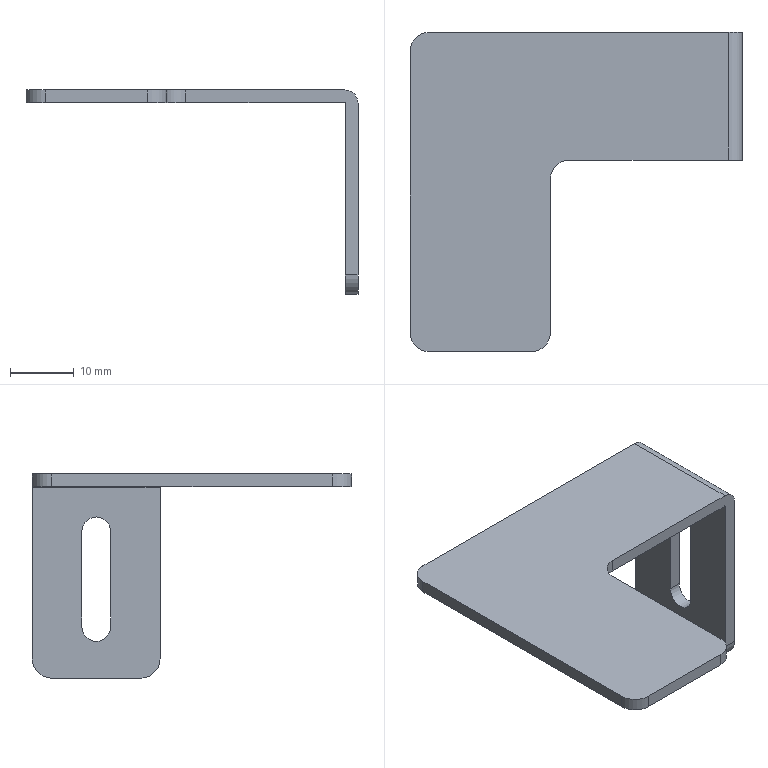Part | SolidWorks | features Fillet 2, Cut 1, FlatPattern 1, ICE 1, SMBaseFlange 1, SheetMetal 1 | 1 solid | 25 faces | box 52 x 50 x 32 mm | volume 4399 mm3 | plane 14 | cylinder 11 | commonest cylinder face diameters 6 x6 4.5 x3 0.2 x1 4.2 x1
STEP:
#1=CARTESIAN_POINT('',(52.,40.,-4.75));
#2=VERTEX_POINT('',#1);
#3=CARTESIAN_POINT('',(52.,42.25,-7.));
#4=VERTEX_POINT('',#3);
#5=CARTESIAN_POINT('',(52.,40.,-7.));
#6=DIRECTION('',(-1.,0.,0.));
#7=DIRECTION('',(0.,0.,1.));
#8=AXIS2_PLACEMENT_3D('',#5,#6,#7);
#9=CIRCLE('',#8,2.25);
#10=EDGE_CURVE('',#2,#4,#9,.T.);
#11=ORIENTED_EDGE('',*,*,#10,.F.);
#12=CARTESIAN_POINT('',(50.,40.,-4.75));
#13=VERTEX_POINT('',#12);
#14=CARTESIAN_POINT('',(52.,40.,-4.75));
#15=DIRECTION('',(-1.,0.,0.));
#16=VECTOR('',#15,1000.);
#17=LINE('',#14,#16);
#18=EDGE_CURVE('',#2,#13,#17,.T.);
#19=ORIENTED_EDGE('',*,*,#18,.T.);
#20=CARTESIAN_POINT('',(50.,42.25,-7.));
#21=VERTEX_POINT('',#20);
#22=CARTESIAN_POINT('',(50.,40.,-7.));
#23=DIRECTION('',(-1.,0.,0.));
#24=DIRECTION('',(0.,0.,1.));
#25=AXIS2_PLACEMENT_3D('',#22,#23,#24);
#26=CIRCLE('',#25,2.25);
#27=EDGE_CURVE('',#13,#21,#26,.T.);
#28=ORIENTED_EDGE('',*,*,#27,.T.);
#29=CARTESIAN_POINT('',(52.,42.25,-7.));
#30=DIRECTION('',(-1.,0.,0.));
#31=VECTOR('',#30,1000.);
#32=LINE('',#29,#31);
#33=EDGE_CURVE('',#4,#21,#32,.T.);
#34=ORIENTED_EDGE('',*,*,#33,.F.);
#35=EDGE_LOOP('',(#11,#19,#28,#34));
#36=FACE_OUTER_BOUND('',#35,.T.);
#37=CARTESIAN_POINT('',(52.,40.,-7.));
#38=DIRECTION('',(-1.,0.,0.));
#39=DIRECTION('',(0.,0.,1.));
#40=AXIS2_PLACEMENT_3D('',#37,#38,#39);
#41=CYLINDRICAL_SURFACE('',#40,2.25);
#42=ADVANCED_FACE('',(#36),#41,.F.);
#43=CARTESIAN_POINT('',(50.,50.,-0.1));
#44=VERTEX_POINT('',#43);
#45=CARTESIAN_POINT('',(52.,50.,-0.1));
#46=VERTEX_POINT('',#45);
#47=CARTESIAN_POINT('',(50.,50.,-0.1));
#48=DIRECTION('',(1.,0.,0.));
#49=VECTOR('',#48,1000.);
#50=LINE('',#47,#49);
#51=EDGE_CURVE('',#44,#46,#50,.T.);
#52=ORIENTED_EDGE('',*,*,#51,.F.);
#53=CARTESIAN_POINT('',(49.9,50.,0.));
#54=VERTEX_POINT('',#53);
#55=CARTESIAN_POINT('',(49.9,50.,-0.1));
#56=DIRECTION('',(0.,1.,0.));
#57=DIRECTION('',(0.,0.,-1.));
#58=AXIS2_PLACEMENT_3D('',#55,#56,#57);
#59=CIRCLE('',#58,0.1);
#60=EDGE_CURVE('',#54,#44,#59,.T.);
#61=ORIENTED_EDGE('',*,*,#60,.F.);
#62=CARTESIAN_POINT('',(49.9,50.,2.));
#63=VERTEX_POINT('',#62);
#64=CARTESIAN_POINT('',(49.9,50.,2.));
#65=DIRECTION('',(0.,0.,-1.));
#66=VECTOR('',#65,1000.);
#67=LINE('',#64,#66);
#68=EDGE_CURVE('',#63,#54,#67,.T.);
#69=ORIENTED_EDGE('',*,*,#68,.F.);
#70=CARTESIAN_POINT('',(49.9,50.,-0.1));
#71=DIRECTION('',(0.,1.,0.));
#72=DIRECTION('',(1.,0.,0.));
#73=AXIS2_PLACEMENT_3D('',#70,#71,#72);
#74=CIRCLE('',#73,2.1);
#75=EDGE_CURVE('',#63,#46,#74,.T.);
#76=ORIENTED_EDGE('',*,*,#75,.T.);
#77=EDGE_LOOP('',(#52,#61,#69,#76));
#78=FACE_OUTER_BOUND('',#77,.T.);
#79=CARTESIAN_POINT('',(50.,50.,-0.1));
#80=DIRECTION('',(0.,1.,0.));
#81=DIRECTION('',(0.,0.,1.));
#82=AXIS2_PLACEMENT_3D('',#79,#80,#81);
#83=PLANE('',#82);
#84=ADVANCED_FACE('',(#78),#83,.T.);
#85=CARTESIAN_POINT('',(52.,50.,-27.));
#86=VERTEX_POINT('',#85);
#87=CARTESIAN_POINT('',(52.,50.,0.));
#88=DIRECTION('',(0.,0.,-1.));
#89=VECTOR('',#88,1000.);
#90=LINE('',#87,#89);
#91=EDGE_CURVE('',#46,#86,#90,.T.);
#92=ORIENTED_EDGE('',*,*,#91,.T.);
#93=CARTESIAN_POINT('',(50.,50.,-27.));
#94=VERTEX_POINT('',#93);
#95=CARTESIAN_POINT('',(49.9,50.,-27.));
#96=DIRECTION('',(-1.,0.,0.));
#97=VECTOR('',#96,1000.);
#98=LINE('',#95,#97);
#99=EDGE_CURVE('',#86,#94,#98,.T.);
#100=ORIENTED_EDGE('',*,*,#99,.T.);
#101=CARTESIAN_POINT('',(50.,50.,0.));
#102=DIRECTION('',(0.,0.,-1.));
#103=VECTOR('',#102,1000.);
#104=LINE('',#101,#103);
#105=EDGE_CURVE('',#44,#94,#104,.T.);
#106=ORIENTED_EDGE('',*,*,#105,.F.);
#107=ORIENTED_EDGE('',*,*,#51,.T.);
#108=EDGE_LOOP('',(#92,#100,#106,#107));
#109=FACE_OUTER_BOUND('',#108,.T.);
#110=CARTESIAN_POINT('',(49.9,50.,2.));
#111=DIRECTION('',(0.,1.,0.));
#112=DIRECTION('',(0.,0.,1.));
#113=AXIS2_PLACEMENT_3D('',#110,#111,#112);
#114=PLANE('',#113);
#115=ADVANCED_FACE('',(#109),#114,.T.);
#116=CARTESIAN_POINT('',(3.,0.,0.));
#117=VERTEX_POINT('',#116);
#118=CARTESIAN_POINT('',(19.,0.,0.));
#119=VERTEX_POINT('',#118);
#120=CARTESIAN_POINT('',(0.,0.,0.));
#121=DIRECTION('',(1.,0.,0.));
#122=VECTOR('',#121,1000.);
#123=LINE('',#120,#122);
#124=EDGE_CURVE('',#117,#119,#123,.T.);
#125=ORIENTED_EDGE('',*,*,#124,.T.);
#126=CARTESIAN_POINT('',(19.,0.,2.));
#127=VERTEX_POINT('',#126);
#128=CARTESIAN_POINT('',(19.,0.,2.));
#129=DIRECTION('',(0.,0.,1.));
#130=VECTOR('',#129,1000.);
#131=LINE('',#128,#130);
#132=EDGE_CURVE('',#119,#127,#131,.T.);
#133=ORIENTED_EDGE('',*,*,#132,.T.);
#134=CARTESIAN_POINT('',(3.,0.,2.));
#135=VERTEX_POINT('',#134);
#136=CARTESIAN_POINT('',(0.,0.,2.));
#137=DIRECTION('',(1.,0.,0.));
#138=VECTOR('',#137,1000.);
#139=LINE('',#136,#138);
#140=EDGE_CURVE('',#135,#127,#139,.T.);
#141=ORIENTED_EDGE('',*,*,#140,.F.);
#142=CARTESIAN_POINT('',(3.,0.,-0.1));
#143=DIRECTION('',(0.,0.,-1.));
#144=VECTOR('',#143,1000.);
#145=LINE('',#142,#144);
#146=EDGE_CURVE('',#135,#117,#145,.T.);
#147=ORIENTED_EDGE('',*,*,#146,.T.);
#148=EDGE_LOOP('',(#125,#133,#141,#147));
#149=FACE_OUTER_BOUND('',#148,.T.);
#150=CARTESIAN_POINT('',(52.,0.,-0.1));
#151=DIRECTION('',(0.,-1.,0.));
#152=DIRECTION('',(0.,0.,-1.));
#153=AXIS2_PLACEMENT_3D('',#150,#151,#152);
#154=PLANE('',#153);
#155=ADVANCED_FACE('',(#149),#154,.T.);
#156=CARTESIAN_POINT('',(52.,37.75,-22.));
#157=VERTEX_POINT('',#156);
#158=CARTESIAN_POINT('',(52.,37.75,-7.));
#159=VERTEX_POINT('',#158);
#160=CARTESIAN_POINT('',(52.,37.75,-7.));
#161=DIRECTION('',(0.,0.,1.));
#162=VECTOR('',#161,1000.);
#163=LINE('',#160,#162);
#164=EDGE_CURVE('',#157,#159,#163,.T.);
#165=ORIENTED_EDGE('',*,*,#164,.T.);
#166=CARTESIAN_POINT('',(52.,40.,-7.));
#167=DIRECTION('',(-1.,0.,0.));
#168=DIRECTION('',(0.,0.,1.));
#169=AXIS2_PLACEMENT_3D('',#166,#167,#168);
#170=CIRCLE('',#169,2.25);
#171=EDGE_CURVE('',#159,#2,#170,.T.);
#172=ORIENTED_EDGE('',*,*,#171,.T.);
#173=ORIENTED_EDGE('',*,*,#10,.T.);
#174=CARTESIAN_POINT('',(52.,42.25,-22.));
#175=VERTEX_POINT('',#174);
#176=CARTESIAN_POINT('',(52.,42.25,-7.));
#177=DIRECTION('',(0.,0.,-1.));
#178=VECTOR('',#177,1000.);
#179=LINE('',#176,#178);
#180=EDGE_CURVE('',#4,#175,#179,.T.);
#181=ORIENTED_EDGE('',*,*,#180,.T.);
#182=CARTESIAN_POINT('',(52.,40.,-22.));
#183=DIRECTION('',(-1.,0.,0.));
#184=DIRECTION('',(0.,0.,1.));
#185=AXIS2_PLACEMENT_3D('',#182,#183,#184);
#186=CIRCLE('',#185,2.25);
#187=EDGE_CURVE('',#175,#157,#186,.T.);
#188=ORIENTED_EDGE('',*,*,#187,.T.);
#189=EDGE_LOOP('',(#165,#172,#173,#181,#188));
#190=FACE_BOUND('',#189,.T.);
#191=CARTESIAN_POINT('',(52.,47.,-30.));
#192=VERTEX_POINT('',#191);
#193=CARTESIAN_POINT('',(52.,33.,-30.));
#194=VERTEX_POINT('',#193);
#195=CARTESIAN_POINT('',(52.,50.,-30.));
#196=DIRECTION('',(0.,-1.,0.));
#197=VECTOR('',#196,1000.);
#198=LINE('',#195,#197);
#199=EDGE_CURVE('',#192,#194,#198,.T.);
#200=ORIENTED_EDGE('',*,*,#199,.F.);
#201=CARTESIAN_POINT('',(52.,47.,-27.));
#202=DIRECTION('',(1.,0.,0.));
#203=DIRECTION('',(0.,0.,1.));
#204=AXIS2_PLACEMENT_3D('',#201,#202,#203);
#205=CIRCLE('',#204,3.);
#206=EDGE_CURVE('',#192,#86,#205,.T.);
#207=ORIENTED_EDGE('',*,*,#206,.T.);
#208=ORIENTED_EDGE('',*,*,#91,.F.);
#209=CARTESIAN_POINT('',(52.,30.,-0.1));
#210=VERTEX_POINT('',#209);
#211=CARTESIAN_POINT('',(52.,50.,-0.1));
#212=DIRECTION('',(0.,-1.,0.));
#213=VECTOR('',#212,1000.);
#214=LINE('',#211,#213);
#215=EDGE_CURVE('',#46,#210,#214,.T.);
#216=ORIENTED_EDGE('',*,*,#215,.T.);
#217=CARTESIAN_POINT('',(52.,30.,-27.));
#218=VERTEX_POINT('',#217);
#219=CARTESIAN_POINT('',(52.,30.,-30.));
#220=DIRECTION('',(0.,0.,1.));
#221=VECTOR('',#220,1000.);
#222=LINE('',#219,#221);
#223=EDGE_CURVE('',#218,#210,#222,.T.);
#224=ORIENTED_EDGE('',*,*,#223,.F.);
#225=CARTESIAN_POINT('',(52.,33.,-27.));
#226=DIRECTION('',(1.,0.,0.));
#227=DIRECTION('',(0.,0.,1.));
#228=AXIS2_PLACEMENT_3D('',#225,#226,#227);
#229=CIRCLE('',#228,3.);
#230=EDGE_CURVE('',#218,#194,#229,.T.);
#231=ORIENTED_EDGE('',*,*,#230,.T.);
#232=EDGE_LOOP('',(#200,#207,#208,#216,#224,#231));
#233=FACE_OUTER_BOUND('',#232,.T.);
#234=CARTESIAN_POINT('',(52.,50.,0.));
#235=DIRECTION('',(-1.,0.,0.));
#236=DIRECTION('',(0.,0.,1.));
#237=AXIS2_PLACEMENT_3D('',#234,#235,#236);
#238=PLANE('',#237);
#239=ADVANCED_FACE('',(#190,#233),#238,.F.);
#240=CARTESIAN_POINT('',(50.,47.,-30.));
#241=VERTEX_POINT('',#240);
#242=CARTESIAN_POINT('',(50.,33.,-30.));
#243=VERTEX_POINT('',#242);
#244=CARTESIAN_POINT('',(50.,50.,-30.));
#245=DIRECTION('',(0.,-1.,0.));
#246=VECTOR('',#245,1000.);
#247=LINE('',#244,#246);
#248=EDGE_CURVE('',#241,#243,#247,.T.);
#249=ORIENTED_EDGE('',*,*,#248,.F.);
#250=CARTESIAN_POINT('',(50.,47.,-30.));
#251=DIRECTION('',(1.,0.,0.));
#252=VECTOR('',#251,1000.);
#253=LINE('',#250,#252);
#254=EDGE_CURVE('',#241,#192,#253,.T.);
#255=ORIENTED_EDGE('',*,*,#254,.T.);
#256=ORIENTED_EDGE('',*,*,#199,.T.);
#257=CARTESIAN_POINT('',(50.,33.,-30.));
#258=DIRECTION('',(-1.,0.,0.));
#259=VECTOR('',#258,1000.);
#260=LINE('',#257,#259);
#261=EDGE_CURVE('',#194,#243,#260,.T.);
#262=ORIENTED_EDGE('',*,*,#261,.T.);
#263=EDGE_LOOP('',(#249,#255,#256,#262));
#264=FACE_OUTER_BOUND('',#263,.T.);
#265=CARTESIAN_POINT('',(50.,50.,-30.));
#266=DIRECTION('',(0.,0.,-1.));
#267=DIRECTION('',(-1.,0.,0.));
#268=AXIS2_PLACEMENT_3D('',#265,#266,#267);
#269=PLANE('',#268);
#270=ADVANCED_FACE('',(#264),#269,.T.);
#271=CARTESIAN_POINT('',(50.,37.75,-7.));
#272=VERTEX_POINT('',#271);
#273=CARTESIAN_POINT('',(50.,40.,-7.));
#274=DIRECTION('',(-1.,0.,0.));
#275=DIRECTION('',(0.,0.,1.));
#276=AXIS2_PLACEMENT_3D('',#273,#274,#275);
#277=CIRCLE('',#276,2.25);
#278=EDGE_CURVE('',#272,#13,#277,.T.);
#279=ORIENTED_EDGE('',*,*,#278,.F.);
#280=CARTESIAN_POINT('',(50.,37.75,-22.));
#281=VERTEX_POINT('',#280);
#282=CARTESIAN_POINT('',(50.,37.75,-7.));
#283=DIRECTION('',(0.,0.,1.));
#284=VECTOR('',#283,1000.);
#285=LINE('',#282,#284);
#286=EDGE_CURVE('',#281,#272,#285,.T.);
#287=ORIENTED_EDGE('',*,*,#286,.F.);
#288=CARTESIAN_POINT('',(50.,42.25,-22.));
#289=VERTEX_POINT('',#288);
#290=CARTESIAN_POINT('',(50.,40.,-22.));
#291=DIRECTION('',(-1.,0.,0.));
#292=DIRECTION('',(0.,0.,1.));
#293=AXIS2_PLACEMENT_3D('',#290,#291,#292);
#294=CIRCLE('',#293,2.25);
#295=EDGE_CURVE('',#289,#281,#294,.T.);
#296=ORIENTED_EDGE('',*,*,#295,.F.);
#297=CARTESIAN_POINT('',(50.,42.25,-7.));
#298=DIRECTION('',(0.,0.,-1.));
#299=VECTOR('',#298,1000.);
#300=LINE('',#297,#299);
#301=EDGE_CURVE('',#21,#289,#300,.T.);
#302=ORIENTED_EDGE('',*,*,#301,.F.);
#303=ORIENTED_EDGE('',*,*,#27,.F.);
#304=EDGE_LOOP('',(#279,#287,#296,#302,#303));
#305=FACE_BOUND('',#304,.T.);
#306=ORIENTED_EDGE('',*,*,#105,.T.);
#307=CARTESIAN_POINT('',(50.,47.,-27.));
#308=DIRECTION('',(-1.,0.,0.));
#309=DIRECTION('',(0.,0.,1.));
#310=AXIS2_PLACEMENT_3D('',#307,#308,#309);
#311=CIRCLE('',#310,3.);
#312=EDGE_CURVE('',#94,#241,#311,.T.);
#313=ORIENTED_EDGE('',*,*,#312,.T.);
#314=ORIENTED_EDGE('',*,*,#248,.T.);
#315=CARTESIAN_POINT('',(50.,30.,-27.));
#316=VERTEX_POINT('',#315);
#317=CARTESIAN_POINT('',(50.,33.,-27.));
#318=DIRECTION('',(-1.,0.,0.));
#319=DIRECTION('',(0.,0.,1.));
#320=AXIS2_PLACEMENT_3D('',#317,#318,#319);
#321=CIRCLE('',#320,3.);
#322=EDGE_CURVE('',#243,#316,#321,.T.);
#323=ORIENTED_EDGE('',*,*,#322,.T.);
#324=CARTESIAN_POINT('',(50.,30.,-0.1));
#325=VERTEX_POINT('',#324);
#326=CARTESIAN_POINT('',(50.,30.,0.));
#327=DIRECTION('',(0.,0.,-1.));
#328=VECTOR('',#327,1000.);
#329=LINE('',#326,#328);
#330=EDGE_CURVE('',#325,#316,#329,.T.);
#331=ORIENTED_EDGE('',*,*,#330,.F.);
#332=CARTESIAN_POINT('',(50.,50.,-0.1));
#333=DIRECTION('',(0.,-1.,0.));
#334=VECTOR('',#333,1000.);
#335=LINE('',#332,#334);
#336=EDGE_CURVE('',#44,#325,#335,.T.);
#337=ORIENTED_EDGE('',*,*,#336,.F.);
#338=EDGE_LOOP('',(#306,#313,#314,#323,#331,#337));
#339=FACE_OUTER_BOUND('',#338,.T.);
#340=CARTESIAN_POINT('',(50.,50.,0.));
#341=DIRECTION('',(-1.,0.,0.));
#342=DIRECTION('',(0.,0.,1.));
#343=AXIS2_PLACEMENT_3D('',#340,#341,#342);
#344=PLANE('',#343);
#345=ADVANCED_FACE('',(#305,#339),#344,.T.);
#346=CARTESIAN_POINT('',(49.9,30.,0.));
#347=VERTEX_POINT('',#346);
#348=CARTESIAN_POINT('',(49.9,30.,-0.1));
#349=DIRECTION('',(0.,1.,0.));
#350=DIRECTION('',(0.,0.,1.));
#351=AXIS2_PLACEMENT_3D('',#348,#349,#350);
#352=CIRCLE('',#351,0.1);
#353=EDGE_CURVE('',#347,#325,#352,.T.);
#354=ORIENTED_EDGE('',*,*,#353,.F.);
#355=CARTESIAN_POINT('',(49.9,50.,0.));
#356=DIRECTION('',(0.,-1.,0.));
#357=VECTOR('',#356,1000.);
#358=LINE('',#355,#357);
#359=EDGE_CURVE('',#54,#347,#358,.T.);
#360=ORIENTED_EDGE('',*,*,#359,.F.);
#361=ORIENTED_EDGE('',*,*,#60,.T.);
#362=ORIENTED_EDGE('',*,*,#336,.T.);
#363=EDGE_LOOP('',(#354,#360,#361,#362));
#364=FACE_OUTER_BOUND('',#363,.T.);
#365=CARTESIAN_POINT('',(49.9,50.,-0.1));
#366=DIRECTION('',(0.,-1.,0.));
#367=DIRECTION('',(0.,0.,-1.));
#368=AXIS2_PLACEMENT_3D('',#365,#366,#367);
#369=CYLINDRICAL_SURFACE('',#368,0.1);
#370=ADVANCED_FACE('',(#364),#369,.F.);
#371=CARTESIAN_POINT('',(0.,47.,0.));
#372=VERTEX_POINT('',#371);
#373=CARTESIAN_POINT('',(0.,3.,0.));
#374=VERTEX_POINT('',#373);
#375=CARTESIAN_POINT('',(0.,50.,0.));
#376=DIRECTION('',(0.,-1.,0.));
#377=VECTOR('',#376,1000.);
#378=LINE('',#375,#377);
#379=EDGE_CURVE('',#372,#374,#378,.T.);
#380=ORIENTED_EDGE('',*,*,#379,.F.);
#381=CARTESIAN_POINT('',(3.,50.,0.));
#382=VERTEX_POINT('',#381);
#383=CARTESIAN_POINT('',(3.,47.,0.));
#384=DIRECTION('',(0.,0.,-1.));
#385=DIRECTION('',(-1.,0.,0.));
#386=AXIS2_PLACEMENT_3D('',#383,#384,#385);
#387=CIRCLE('',#386,3.);
#388=EDGE_CURVE('',#372,#382,#387,.T.);
#389=ORIENTED_EDGE('',*,*,#388,.T.);
#390=CARTESIAN_POINT('',(0.,50.,0.));
#391=DIRECTION('',(1.,0.,0.));
#392=VECTOR('',#391,1000.);
#393=LINE('',#390,#392);
#394=EDGE_CURVE('',#382,#54,#393,.T.);
#395=ORIENTED_EDGE('',*,*,#394,.T.);
#396=ORIENTED_EDGE('',*,*,#359,.T.);
#397=CARTESIAN_POINT('',(25.,30.,0.));
#398=VERTEX_POINT('',#397);
#399=CARTESIAN_POINT('',(0.,30.,0.));
#400=DIRECTION('',(1.,0.,0.));
#401=VECTOR('',#400,1000.);
#402=LINE('',#399,#401);
#403=EDGE_CURVE('',#398,#347,#402,.T.);
#404=ORIENTED_EDGE('',*,*,#403,.F.);
#405=CARTESIAN_POINT('',(22.,27.,0.));
#406=VERTEX_POINT('',#405);
#407=CARTESIAN_POINT('',(25.,27.,0.));
#408=DIRECTION('',(0.,0.,1.));
#409=DIRECTION('',(-1.,0.,0.));
#410=AXIS2_PLACEMENT_3D('',#407,#408,#409);
#411=CIRCLE('',#410,3.);
#412=EDGE_CURVE('',#398,#406,#411,.T.);
#413=ORIENTED_EDGE('',*,*,#412,.T.);
#414=CARTESIAN_POINT('',(22.,3.,0.));
#415=VERTEX_POINT('',#414);
#416=CARTESIAN_POINT('',(22.,50.,0.));
#417=DIRECTION('',(0.,1.,0.));
#418=VECTOR('',#417,1000.);
#419=LINE('',#416,#418);
#420=EDGE_CURVE('',#415,#406,#419,.T.);
#421=ORIENTED_EDGE('',*,*,#420,.F.);
#422=CARTESIAN_POINT('',(19.,3.,0.));
#423=DIRECTION('',(0.,0.,-1.));
#424=DIRECTION('',(-1.,0.,0.));
#425=AXIS2_PLACEMENT_3D('',#422,#423,#424);
#426=CIRCLE('',#425,3.);
#427=EDGE_CURVE('',#415,#119,#426,.T.);
#428=ORIENTED_EDGE('',*,*,#427,.T.);
#429=ORIENTED_EDGE('',*,*,#124,.F.);
#430=CARTESIAN_POINT('',(3.,3.,0.));
#431=DIRECTION('',(0.,0.,-1.));
#432=DIRECTION('',(-1.,0.,0.));
#433=AXIS2_PLACEMENT_3D('',#430,#431,#432);
#434=CIRCLE('',#433,3.);
#435=EDGE_CURVE('',#117,#374,#434,.T.);
#436=ORIENTED_EDGE('',*,*,#435,.T.);
#437=EDGE_LOOP('',(#380,#389,#395,#396,#404,#413,#421,#428,#429,#436));
#438=FACE_OUTER_BOUND('',#437,.T.);
#439=CARTESIAN_POINT('',(0.,50.,0.));
#440=DIRECTION('',(0.,0.,-1.));
#441=DIRECTION('',(-1.,0.,0.));
#442=AXIS2_PLACEMENT_3D('',#439,#440,#441);
#443=PLANE('',#442);
#444=ADVANCED_FACE('',(#438),#443,.T.);
#445=CARTESIAN_POINT('',(0.,47.,2.));
#446=VERTEX_POINT('',#445);
#447=CARTESIAN_POINT('',(0.,3.,2.));
#448=VERTEX_POINT('',#447);
#449=CARTESIAN_POINT('',(0.,50.,2.));
#450=DIRECTION('',(0.,-1.,0.));
#451=VECTOR('',#450,1000.);
#452=LINE('',#449,#451);
#453=EDGE_CURVE('',#446,#448,#452,.T.);
#454=ORIENTED_EDGE('',*,*,#453,.F.);
#455=CARTESIAN_POINT('',(0.,47.,0.));
#456=DIRECTION('',(0.,0.,-1.));
#457=VECTOR('',#456,1000.);
#458=LINE('',#455,#457);
#459=EDGE_CURVE('',#446,#372,#458,.T.);
#460=ORIENTED_EDGE('',*,*,#459,.T.);
#461=ORIENTED_EDGE('',*,*,#379,.T.);
#462=CARTESIAN_POINT('',(0.,3.,2.));
#463=DIRECTION('',(0.,0.,1.));
#464=VECTOR('',#463,1000.);
#465=LINE('',#462,#464);
#466=EDGE_CURVE('',#374,#448,#465,.T.);
#467=ORIENTED_EDGE('',*,*,#466,.T.);
#468=EDGE_LOOP('',(#454,#460,#461,#467));
#469=FACE_OUTER_BOUND('',#468,.T.);
#470=CARTESIAN_POINT('',(0.,50.,2.));
#471=DIRECTION('',(-1.,0.,0.));
#472=DIRECTION('',(0.,0.,1.));
#473=AXIS2_PLACEMENT_3D('',#470,#471,#472);
#474=PLANE('',#473);
#475=ADVANCED_FACE('',(#469),#474,.T.);
#476=CARTESIAN_POINT('',(3.,50.,2.));
#477=VERTEX_POINT('',#476);
#478=CARTESIAN_POINT('',(0.,50.,2.));
#479=DIRECTION('',(1.,0.,0.));
#480=VECTOR('',#479,1000.);
#481=LINE('',#478,#480);
#482=EDGE_CURVE('',#477,#63,#481,.T.);
#483=ORIENTED_EDGE('',*,*,#482,.F.);
#484=CARTESIAN_POINT('',(3.,47.,2.));
#485=DIRECTION('',(0.,0.,1.));
#486=DIRECTION('',(-1.,0.,0.));
#487=AXIS2_PLACEMENT_3D('',#484,#485,#486);
#488=CIRCLE('',#487,3.);
#489=EDGE_CURVE('',#477,#446,#488,.T.);
#490=ORIENTED_EDGE('',*,*,#489,.T.);
#491=ORIENTED_EDGE('',*,*,#453,.T.);
#492=CARTESIAN_POINT('',(3.,3.,2.));
#493=DIRECTION('',(0.,0.,1.));
#494=DIRECTION('',(-1.,0.,0.));
#495=AXIS2_PLACEMENT_3D('',#492,#493,#494);
#496=CIRCLE('',#495,3.);
#497=EDGE_CURVE('',#448,#135,#496,.T.);
#498=ORIENTED_EDGE('',*,*,#497,.T.);
#499=ORIENTED_EDGE('',*,*,#140,.T.);
#500=CARTESIAN_POINT('',(22.,3.,2.));
#501=VERTEX_POINT('',#500);
#502=CARTESIAN_POINT('',(19.,3.,2.));
#503=DIRECTION('',(0.,0.,1.));
#504=DIRECTION('',(-1.,0.,0.));
#505=AXIS2_PLACEMENT_3D('',#502,#503,#504);
#506=CIRCLE('',#505,3.);
#507=EDGE_CURVE('',#127,#501,#506,.T.);
#508=ORIENTED_EDGE('',*,*,#507,.T.);
#509=CARTESIAN_POINT('',(22.,27.,2.));
#510=VERTEX_POINT('',#509);
#511=CARTESIAN_POINT('',(22.,0.,2.));
#512=DIRECTION('',(0.,-1.,0.));
#513=VECTOR('',#512,1000.);
#514=LINE('',#511,#513);
#515=EDGE_CURVE('',#510,#501,#514,.T.);
#516=ORIENTED_EDGE('',*,*,#515,.F.);
#517=CARTESIAN_POINT('',(25.,30.,2.));
#518=VERTEX_POINT('',#517);
#519=CARTESIAN_POINT('',(25.,27.,2.));
#520=DIRECTION('',(0.,0.,-1.));
#521=DIRECTION('',(-1.,0.,0.));
#522=AXIS2_PLACEMENT_3D('',#519,#520,#521);
#523=CIRCLE('',#522,3.);
#524=EDGE_CURVE('',#510,#518,#523,.T.);
#525=ORIENTED_EDGE('',*,*,#524,.T.);
#526=CARTESIAN_POINT('',(49.9,30.,2.));
#527=VERTEX_POINT('',#526);
#528=CARTESIAN_POINT('',(22.,30.,2.));
#529=DIRECTION('',(-1.,0.,0.));
#530=VECTOR('',#529,1000.);
#531=LINE('',#528,#530);
#532=EDGE_CURVE('',#527,#518,#531,.T.);
#533=ORIENTED_EDGE('',*,*,#532,.F.);
#534=CARTESIAN_POINT('',(49.9,50.,2.));
#535=DIRECTION('',(0.,-1.,0.));
#536=VECTOR('',#535,1000.);
#537=LINE('',#534,#536);
#538=EDGE_CURVE('',#63,#527,#537,.T.);
#539=ORIENTED_EDGE('',*,*,#538,.F.);
#540=EDGE_LOOP('',(#483,#490,#491,#498,#499,#508,#516,#525,#533,#539));
#541=FACE_OUTER_BOUND('',#540,.T.);
#542=CARTESIAN_POINT('',(0.,50.,2.));
#543=DIRECTION('',(0.,0.,-1.));
#544=DIRECTION('',(-1.,0.,0.));
#545=AXIS2_PLACEMENT_3D('',#542,#543,#544);
#546=PLANE('',#545);
#547=ADVANCED_FACE('',(#541),#546,.F.);
#548=ORIENTED_EDGE('',*,*,#538,.T.);
#549=CARTESIAN_POINT('',(49.9,30.,-0.1));
#550=DIRECTION('',(0.,1.,0.));
#551=DIRECTION('',(0.,0.,1.));
#552=AXIS2_PLACEMENT_3D('',#549,#550,#551);
#553=CIRCLE('',#552,2.1);
#554=EDGE_CURVE('',#527,#210,#553,.T.);
#555=ORIENTED_EDGE('',*,*,#554,.T.);
#556=ORIENTED_EDGE('',*,*,#215,.F.);
#557=ORIENTED_EDGE('',*,*,#75,.F.);
#558=EDGE_LOOP('',(#548,#555,#556,#557));
#559=FACE_OUTER_BOUND('',#558,.T.);
#560=CARTESIAN_POINT('',(49.9,50.,-0.1));
#561=DIRECTION('',(0.,-1.,0.));
#562=DIRECTION('',(0.,0.,-1.));
#563=AXIS2_PLACEMENT_3D('',#560,#561,#562);
#564=CYLINDRICAL_SURFACE('',#563,2.1);
#565=ADVANCED_FACE('',(#559),#564,.T.);
#566=ORIENTED_EDGE('',*,*,#394,.F.);
#567=CARTESIAN_POINT('',(3.,50.,2.));
#568=DIRECTION('',(0.,0.,1.));
#569=VECTOR('',#568,1000.);
#570=LINE('',#567,#569);
#571=EDGE_CURVE('',#382,#477,#570,.T.);
#572=ORIENTED_EDGE('',*,*,#571,.T.);
#573=ORIENTED_EDGE('',*,*,#482,.T.);
#574=ORIENTED_EDGE('',*,*,#68,.T.);
#575=EDGE_LOOP('',(#566,#572,#573,#574));
#576=FACE_OUTER_BOUND('',#575,.T.);
#577=CARTESIAN_POINT('',(49.9,50.,-0.1));
#578=DIRECTION('',(0.,-1.,0.));
#579=DIRECTION('',(-1.,0.,0.));
#580=AXIS2_PLACEMENT_3D('',#577,#578,#579);
#581=PLANE('',#580);
#582=ADVANCED_FACE('',(#576),#581,.F.);
#583=ORIENTED_EDGE('',*,*,#330,.T.);
#584=CARTESIAN_POINT('',(52.,30.,-27.));
#585=DIRECTION('',(1.,0.,0.));
#586=VECTOR('',#585,1000.);
#587=LINE('',#584,#586);
#588=EDGE_CURVE('',#316,#218,#587,.T.);
#589=ORIENTED_EDGE('',*,*,#588,.T.);
#590=ORIENTED_EDGE('',*,*,#223,.T.);
#591=ORIENTED_EDGE('',*,*,#554,.F.);
#592=ORIENTED_EDGE('',*,*,#532,.T.);
#593=CARTESIAN_POINT('',(25.,30.,0.));
#594=DIRECTION('',(0.,0.,-1.));
#595=VECTOR('',#594,1000.);
#596=LINE('',#593,#595);
#597=EDGE_CURVE('',#518,#398,#596,.T.);
#598=ORIENTED_EDGE('',*,*,#597,.T.);
#599=ORIENTED_EDGE('',*,*,#403,.T.);
#600=ORIENTED_EDGE('',*,*,#353,.T.);
#601=EDGE_LOOP('',(#583,#589,#590,#591,#592,#598,#599,#600));
#602=FACE_OUTER_BOUND('',#601,.T.);
#603=CARTESIAN_POINT('',(22.,30.,-30.));
#604=DIRECTION('',(0.,1.,0.));
#605=DIRECTION('',(0.,0.,1.));
#606=AXIS2_PLACEMENT_3D('',#603,#604,#605);
#607=PLANE('',#606);
#608=ADVANCED_FACE('',(#602),#607,.F.);
#609=ORIENTED_EDGE('',*,*,#420,.T.);
#610=CARTESIAN_POINT('',(22.,27.,2.));
#611=DIRECTION('',(0.,0.,1.));
#612=VECTOR('',#611,1000.);
#613=LINE('',#610,#612);
#614=EDGE_CURVE('',#406,#510,#613,.T.);
#615=ORIENTED_EDGE('',*,*,#614,.T.);
#616=ORIENTED_EDGE('',*,*,#515,.T.);
#617=CARTESIAN_POINT('',(22.,3.,0.));
#618=DIRECTION('',(0.,0.,-1.));
#619=VECTOR('',#618,1000.);
#620=LINE('',#617,#619);
#621=EDGE_CURVE('',#501,#415,#620,.T.);
#622=ORIENTED_EDGE('',*,*,#621,.T.);
#623=EDGE_LOOP('',(#609,#615,#616,#622));
#624=FACE_OUTER_BOUND('',#623,.T.);
#625=CARTESIAN_POINT('',(22.,0.,-30.));
#626=DIRECTION('',(-1.,0.,0.));
#627=DIRECTION('',(0.,0.,1.));
#628=AXIS2_PLACEMENT_3D('',#625,#626,#627);
#629=PLANE('',#628);
#630=ADVANCED_FACE('',(#624),#629,.F.);
#631=ORIENTED_EDGE('',*,*,#18,.F.);
#632=ORIENTED_EDGE('',*,*,#171,.F.);
#633=CARTESIAN_POINT('',(52.,37.75,-7.));
#634=DIRECTION('',(-1.,0.,0.));
#635=VECTOR('',#634,1000.);
#636=LINE('',#633,#635);
#637=EDGE_CURVE('',#159,#272,#636,.T.);
#638=ORIENTED_EDGE('',*,*,#637,.T.);
#639=ORIENTED_EDGE('',*,*,#278,.T.);
#640=EDGE_LOOP('',(#631,#632,#638,#639));
#641=FACE_OUTER_BOUND('',#640,.T.);
#642=CARTESIAN_POINT('',(52.,40.,-7.));
#643=DIRECTION('',(-1.,0.,0.));
#644=DIRECTION('',(0.,0.,1.));
#645=AXIS2_PLACEMENT_3D('',#642,#643,#644);
#646=CYLINDRICAL_SURFACE('',#645,2.25);
#647=ADVANCED_FACE('',(#641),#646,.F.);
#648=ORIENTED_EDGE('',*,*,#286,.T.);
#649=ORIENTED_EDGE('',*,*,#637,.F.);
#650=ORIENTED_EDGE('',*,*,#164,.F.);
#651=CARTESIAN_POINT('',(52.,37.75,-22.));
#652=DIRECTION('',(-1.,0.,0.));
#653=VECTOR('',#652,1000.);
#654=LINE('',#651,#653);
#655=EDGE_CURVE('',#157,#281,#654,.T.);
#656=ORIENTED_EDGE('',*,*,#655,.T.);
#657=EDGE_LOOP('',(#648,#649,#650,#656));
#658=FACE_OUTER_BOUND('',#657,.T.);
#659=CARTESIAN_POINT('',(52.,37.75,-7.));
#660=DIRECTION('',(0.,-1.,0.));
#661=DIRECTION('',(0.,0.,-1.));
#662=AXIS2_PLACEMENT_3D('',#659,#660,#661);
#663=PLANE('',#662);
#664=ADVANCED_FACE('',(#658),#663,.F.);
#665=ORIENTED_EDGE('',*,*,#295,.T.);
#666=ORIENTED_EDGE('',*,*,#655,.F.);
#667=ORIENTED_EDGE('',*,*,#187,.F.);
#668=CARTESIAN_POINT('',(52.,42.25,-22.));
#669=DIRECTION('',(-1.,0.,0.));
#670=VECTOR('',#669,1000.);
#671=LINE('',#668,#670);
#672=EDGE_CURVE('',#175,#289,#671,.T.);
#673=ORIENTED_EDGE('',*,*,#672,.T.);
#674=EDGE_LOOP('',(#665,#666,#667,#673));
#675=FACE_OUTER_BOUND('',#674,.T.);
#676=CARTESIAN_POINT('',(52.,40.,-22.));
#677=DIRECTION('',(-1.,0.,0.));
#678=DIRECTION('',(0.,0.,1.));
#679=AXIS2_PLACEMENT_3D('',#676,#677,#678);
#680=CYLINDRICAL_SURFACE('',#679,2.25);
#681=ADVANCED_FACE('',(#675),#680,.F.);
#682=ORIENTED_EDGE('',*,*,#301,.T.);
#683=ORIENTED_EDGE('',*,*,#672,.F.);
#684=ORIENTED_EDGE('',*,*,#180,.F.);
#685=ORIENTED_EDGE('',*,*,#33,.T.);
#686=EDGE_LOOP('',(#682,#683,#684,#685));
#687=FACE_OUTER_BOUND('',#686,.T.);
#688=CARTESIAN_POINT('',(52.,42.25,-7.));
#689=DIRECTION('',(0.,1.,0.));
#690=DIRECTION('',(0.,0.,1.));
#691=AXIS2_PLACEMENT_3D('',#688,#689,#690);
#692=PLANE('',#691);
#693=ADVANCED_FACE('',(#687),#692,.F.);
#694=ORIENTED_EDGE('',*,*,#489,.F.);
#695=ORIENTED_EDGE('',*,*,#571,.F.);
#696=ORIENTED_EDGE('',*,*,#388,.F.);
#697=ORIENTED_EDGE('',*,*,#459,.F.);
#698=EDGE_LOOP('',(#694,#695,#696,#697));
#699=FACE_OUTER_BOUND('',#698,.T.);
#700=CARTESIAN_POINT('',(3.,47.,2.));
#701=DIRECTION('',(0.,0.,1.));
#702=DIRECTION('',(1.,0.,0.));
#703=AXIS2_PLACEMENT_3D('',#700,#701,#702);
#704=CYLINDRICAL_SURFACE('',#703,3.);
#705=ADVANCED_FACE('',(#699),#704,.T.);
#706=ORIENTED_EDGE('',*,*,#412,.F.);
#707=ORIENTED_EDGE('',*,*,#597,.F.);
#708=ORIENTED_EDGE('',*,*,#524,.F.);
#709=ORIENTED_EDGE('',*,*,#614,.F.);
#710=EDGE_LOOP('',(#706,#707,#708,#709));
#711=FACE_OUTER_BOUND('',#710,.T.);
#712=CARTESIAN_POINT('',(25.,27.,-30.));
#713=DIRECTION('',(0.,0.,-1.));
#714=DIRECTION('',(-1.,0.,0.));
#715=AXIS2_PLACEMENT_3D('',#712,#713,#714);
#716=CYLINDRICAL_SURFACE('',#715,3.);
#717=ADVANCED_FACE('',(#711),#716,.F.);
#718=ORIENTED_EDGE('',*,*,#427,.F.);
#719=ORIENTED_EDGE('',*,*,#621,.F.);
#720=ORIENTED_EDGE('',*,*,#507,.F.);
#721=ORIENTED_EDGE('',*,*,#132,.F.);
#722=EDGE_LOOP('',(#718,#719,#720,#721));
#723=FACE_OUTER_BOUND('',#722,.T.);
#724=CARTESIAN_POINT('',(19.,3.,-0.1));
#725=DIRECTION('',(0.,0.,-1.));
#726=DIRECTION('',(-1.,0.,0.));
#727=AXIS2_PLACEMENT_3D('',#724,#725,#726);
#728=CYLINDRICAL_SURFACE('',#727,3.);
#729=ADVANCED_FACE('',(#723),#728,.T.);
#730=ORIENTED_EDGE('',*,*,#497,.F.);
#731=ORIENTED_EDGE('',*,*,#466,.F.);
#732=ORIENTED_EDGE('',*,*,#435,.F.);
#733=ORIENTED_EDGE('',*,*,#146,.F.);
#734=EDGE_LOOP('',(#730,#731,#732,#733));
#735=FACE_OUTER_BOUND('',#734,.T.);
#736=CARTESIAN_POINT('',(3.,3.,-0.1));
#737=DIRECTION('',(0.,0.,-1.));
#738=DIRECTION('',(-1.,0.,0.));
#739=AXIS2_PLACEMENT_3D('',#736,#737,#738);
#740=CYLINDRICAL_SURFACE('',#739,3.);
#741=ADVANCED_FACE('',(#735),#740,.T.);
#742=ORIENTED_EDGE('',*,*,#312,.F.);
#743=ORIENTED_EDGE('',*,*,#99,.F.);
#744=ORIENTED_EDGE('',*,*,#206,.F.);
#745=ORIENTED_EDGE('',*,*,#254,.F.);
#746=EDGE_LOOP('',(#742,#743,#744,#745));
#747=FACE_OUTER_BOUND('',#746,.T.);
#748=CARTESIAN_POINT('',(50.,47.,-27.));
#749=DIRECTION('',(1.,0.,0.));
#750=DIRECTION('',(0.,0.,-1.));
#751=AXIS2_PLACEMENT_3D('',#748,#749,#750);
#752=CYLINDRICAL_SURFACE('',#751,3.);
#753=ADVANCED_FACE('',(#747),#752,.T.);
#754=ORIENTED_EDGE('',*,*,#230,.F.);
#755=ORIENTED_EDGE('',*,*,#588,.F.);
#756=ORIENTED_EDGE('',*,*,#322,.F.);
#757=ORIENTED_EDGE('',*,*,#261,.F.);
#758=EDGE_LOOP('',(#754,#755,#756,#757));
#759=FACE_OUTER_BOUND('',#758,.T.);
#760=CARTESIAN_POINT('',(50.,33.,-27.));
#761=DIRECTION('',(1.,0.,0.));
#762=DIRECTION('',(0.,0.,-1.));
#763=AXIS2_PLACEMENT_3D('',#760,#761,#762);
#764=CYLINDRICAL_SURFACE('',#763,3.);
#765=ADVANCED_FACE('',(#759),#764,.T.);
#766=CLOSED_SHELL('',(#42,#84,#115,#155,#239,#270,#345,#370,#444,#475,#547,#565,#582,#608,#630,#647,#664,#681,#693,#705,#717,#729,#741,#753,#765));
#767=MANIFOLD_SOLID_BREP('',#766);
#768=CARTESIAN_POINT('',(0.,0.,0.));
#769=DIRECTION('',(0.,0.,1.));
#770=DIRECTION('',(1.,0.,0.));
#771=AXIS2_PLACEMENT_3D('',#768,#769,#770);
#772=(LENGTH_UNIT()NAMED_UNIT(*)SI_UNIT(.MILLI.,.METRE.));
#773=UNCERTAINTY_MEASURE_WITH_UNIT(LENGTH_MEASURE(0.00001),#772,'','');
#774=(NAMED_UNIT(*)PLANE_ANGLE_UNIT()SI_UNIT($,.RADIAN.));
#775=(NAMED_UNIT(*)SI_UNIT($,.STERADIAN.)SOLID_ANGLE_UNIT());
#776=(GEOMETRIC_REPRESENTATION_CONTEXT(3)GLOBAL_UNCERTAINTY_ASSIGNED_CONTEXT((#773))GLOBAL_UNIT_ASSIGNED_CONTEXT((#772,#774,#775))REPRESENTATION_CONTEXT('',''));
#777=ADVANCED_BREP_SHAPE_REPRESENTATION('',(#767,#771),#776);